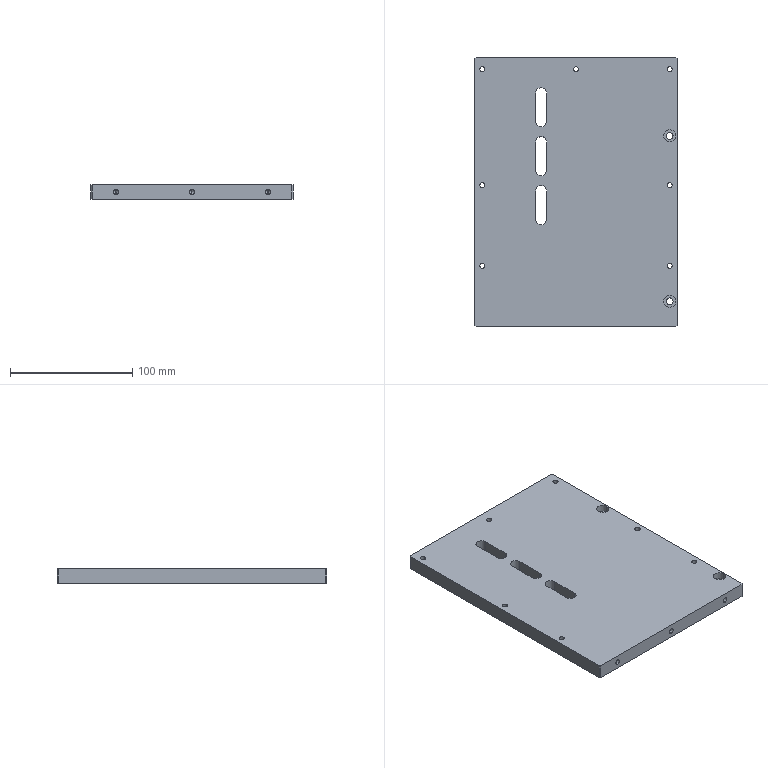Part | SolidWorks | features HoleWzd 4, Chamfer 1, Extrusion 1, Fillet 1, ICE 1 | 1 solid | 64 faces | box 165 x 220.4 x 12 mm | volume 385919 mm3 | cylinder 36 | plane 22 | cone 6 | commonest cylinder face diameters 4.2 x20 9 x6 5.5 x4 10 x4 6 x2